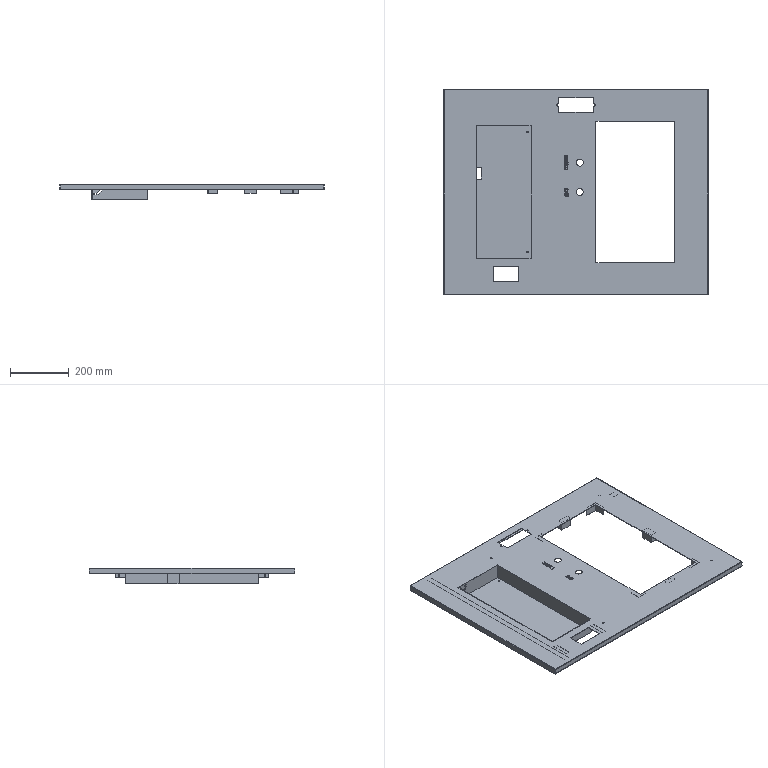Part | STEP file | NX21001-08-MA-02-003-001-DM2r | 1 solid | 501 faces | box 900 x 700 x 54 mm | volume 1485136 mm3 | plane 261 | spline 137 | cylinder 83 | cone 12 | sphere 8 | commonest cylinder face diameters 4 x18 6 x18 4.2 x16 3.3 x14 23 x8 7 x3